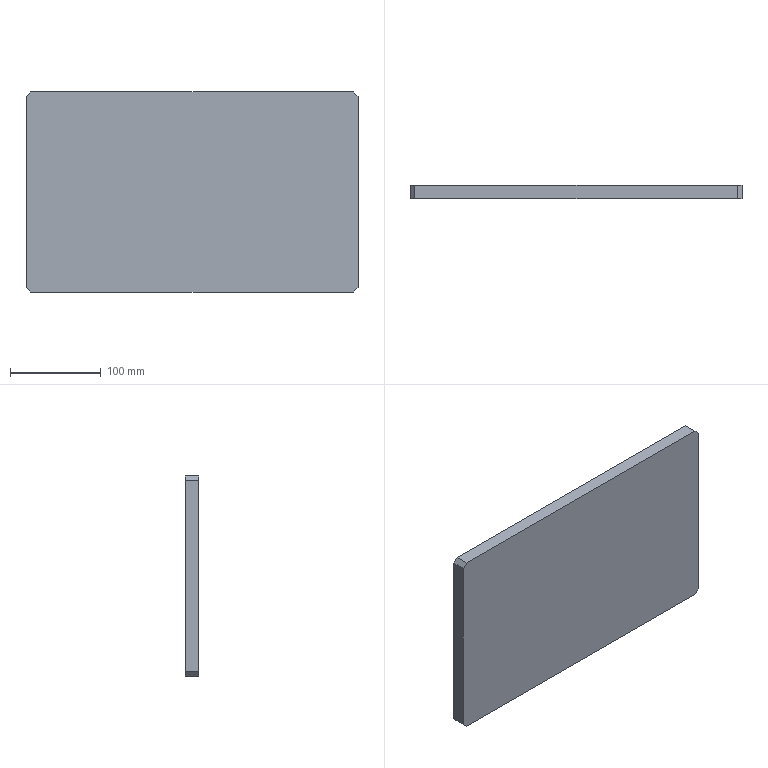Part | SolidWorks | features BaseBody 1 | 1 solid | 10 faces | box 365 x 15 x 220 mm | volume 1203750 mm3 | plane 10
STEP:
#1=CARTESIAN_POINT('',(360.,15.,-220.));
#2=VERTEX_POINT('',#1);
#3=CARTESIAN_POINT('',(365.,15.,-215.));
#4=VERTEX_POINT('',#3);
#5=CARTESIAN_POINT('',(360.,15.,-220.));
#6=DIRECTION('',(0.7071,0.,0.7071));
#7=VECTOR('',#6,1000.);
#8=LINE('',#5,#7);
#9=EDGE_CURVE('',#2,#4,#8,.T.);
#10=ORIENTED_EDGE('',*,*,#9,.F.);
#11=CARTESIAN_POINT('',(5.,15.,-220.));
#12=VERTEX_POINT('',#11);
#13=CARTESIAN_POINT('',(0.,15.,-220.));
#14=DIRECTION('',(1.,0.,0.));
#15=VECTOR('',#14,1000.);
#16=LINE('',#13,#15);
#17=EDGE_CURVE('',#12,#2,#16,.T.);
#18=ORIENTED_EDGE('',*,*,#17,.F.);
#19=CARTESIAN_POINT('',(0.,15.,-215.));
#20=VERTEX_POINT('',#19);
#21=CARTESIAN_POINT('',(0.,15.,-215.));
#22=DIRECTION('',(0.7071,0.,-0.7071));
#23=VECTOR('',#22,1000.);
#24=LINE('',#21,#23);
#25=EDGE_CURVE('',#20,#12,#24,.T.);
#26=ORIENTED_EDGE('',*,*,#25,.F.);
#27=CARTESIAN_POINT('',(0.,15.,-5.));
#28=VERTEX_POINT('',#27);
#29=CARTESIAN_POINT('',(0.,15.,0.));
#30=DIRECTION('',(0.,0.,-1.));
#31=VECTOR('',#30,1000.);
#32=LINE('',#29,#31);
#33=EDGE_CURVE('',#28,#20,#32,.T.);
#34=ORIENTED_EDGE('',*,*,#33,.F.);
#35=CARTESIAN_POINT('',(5.,15.,0.));
#36=VERTEX_POINT('',#35);
#37=CARTESIAN_POINT('',(5.,15.,0.));
#38=DIRECTION('',(-0.7071,0.,-0.7071));
#39=VECTOR('',#38,1000.);
#40=LINE('',#37,#39);
#41=EDGE_CURVE('',#36,#28,#40,.T.);
#42=ORIENTED_EDGE('',*,*,#41,.F.);
#43=CARTESIAN_POINT('',(360.,15.,0.));
#44=VERTEX_POINT('',#43);
#45=CARTESIAN_POINT('',(0.,15.,0.));
#46=DIRECTION('',(-1.,0.,0.));
#47=VECTOR('',#46,1000.);
#48=LINE('',#45,#47);
#49=EDGE_CURVE('',#44,#36,#48,.T.);
#50=ORIENTED_EDGE('',*,*,#49,.F.);
#51=CARTESIAN_POINT('',(365.,15.,-5.));
#52=VERTEX_POINT('',#51);
#53=CARTESIAN_POINT('',(365.,15.,-5.));
#54=DIRECTION('',(-0.7071,0.,0.7071));
#55=VECTOR('',#54,1000.);
#56=LINE('',#53,#55);
#57=EDGE_CURVE('',#52,#44,#56,.T.);
#58=ORIENTED_EDGE('',*,*,#57,.F.);
#59=CARTESIAN_POINT('',(365.,15.,0.));
#60=DIRECTION('',(0.,0.,1.));
#61=VECTOR('',#60,1000.);
#62=LINE('',#59,#61);
#63=EDGE_CURVE('',#4,#52,#62,.T.);
#64=ORIENTED_EDGE('',*,*,#63,.F.);
#65=EDGE_LOOP('',(#10,#18,#26,#34,#42,#50,#58,#64));
#66=FACE_OUTER_BOUND('',#65,.T.);
#67=CARTESIAN_POINT('',(0.,15.,0.));
#68=DIRECTION('',(0.,-1.,0.));
#69=DIRECTION('',(0.,0.,-1.));
#70=AXIS2_PLACEMENT_3D('',#67,#68,#69);
#71=PLANE('',#70);
#72=ADVANCED_FACE('',(#66),#71,.F.);
#73=CARTESIAN_POINT('',(365.,0.,-215.));
#74=VERTEX_POINT('',#73);
#75=CARTESIAN_POINT('',(365.,15.,-215.));
#76=DIRECTION('',(0.,-1.,0.));
#77=VECTOR('',#76,1000.);
#78=LINE('',#75,#77);
#79=EDGE_CURVE('',#4,#74,#78,.T.);
#80=ORIENTED_EDGE('',*,*,#79,.F.);
#81=ORIENTED_EDGE('',*,*,#63,.T.);
#82=CARTESIAN_POINT('',(365.,0.,-5.));
#83=VERTEX_POINT('',#82);
#84=CARTESIAN_POINT('',(365.,15.,-5.));
#85=DIRECTION('',(0.,1.,0.));
#86=VECTOR('',#85,1000.);
#87=LINE('',#84,#86);
#88=EDGE_CURVE('',#83,#52,#87,.T.);
#89=ORIENTED_EDGE('',*,*,#88,.F.);
#90=CARTESIAN_POINT('',(365.,0.,0.));
#91=DIRECTION('',(0.,0.,1.));
#92=VECTOR('',#91,1000.);
#93=LINE('',#90,#92);
#94=EDGE_CURVE('',#74,#83,#93,.T.);
#95=ORIENTED_EDGE('',*,*,#94,.F.);
#96=EDGE_LOOP('',(#80,#81,#89,#95));
#97=FACE_OUTER_BOUND('',#96,.T.);
#98=CARTESIAN_POINT('',(365.,15.,0.));
#99=DIRECTION('',(-1.,0.,0.));
#100=DIRECTION('',(0.,0.,1.));
#101=AXIS2_PLACEMENT_3D('',#98,#99,#100);
#102=PLANE('',#101);
#103=ADVANCED_FACE('',(#97),#102,.F.);
#104=ORIENTED_EDGE('',*,*,#79,.T.);
#105=CARTESIAN_POINT('',(360.,0.,-220.));
#106=VERTEX_POINT('',#105);
#107=CARTESIAN_POINT('',(360.,0.,-220.));
#108=DIRECTION('',(0.7071,0.,0.7071));
#109=VECTOR('',#108,1000.);
#110=LINE('',#107,#109);
#111=EDGE_CURVE('',#106,#74,#110,.T.);
#112=ORIENTED_EDGE('',*,*,#111,.F.);
#113=CARTESIAN_POINT('',(360.,15.,-220.));
#114=DIRECTION('',(0.,-1.,0.));
#115=VECTOR('',#114,1000.);
#116=LINE('',#113,#115);
#117=EDGE_CURVE('',#2,#106,#116,.T.);
#118=ORIENTED_EDGE('',*,*,#117,.F.);
#119=ORIENTED_EDGE('',*,*,#9,.T.);
#120=EDGE_LOOP('',(#104,#112,#118,#119));
#121=FACE_OUTER_BOUND('',#120,.T.);
#122=CARTESIAN_POINT('',(360.,15.,-220.));
#123=DIRECTION('',(-0.7071,0.,0.7071));
#124=DIRECTION('',(0.7071,0.,0.7071));
#125=AXIS2_PLACEMENT_3D('',#122,#123,#124);
#126=PLANE('',#125);
#127=ADVANCED_FACE('',(#121),#126,.F.);
#128=ORIENTED_EDGE('',*,*,#117,.T.);
#129=CARTESIAN_POINT('',(5.,0.,-220.));
#130=VERTEX_POINT('',#129);
#131=CARTESIAN_POINT('',(0.,0.,-220.));
#132=DIRECTION('',(1.,0.,0.));
#133=VECTOR('',#132,1000.);
#134=LINE('',#131,#133);
#135=EDGE_CURVE('',#130,#106,#134,.T.);
#136=ORIENTED_EDGE('',*,*,#135,.F.);
#137=CARTESIAN_POINT('',(5.,15.,-220.));
#138=DIRECTION('',(0.,-1.,0.));
#139=VECTOR('',#138,1000.);
#140=LINE('',#137,#139);
#141=EDGE_CURVE('',#12,#130,#140,.T.);
#142=ORIENTED_EDGE('',*,*,#141,.F.);
#143=ORIENTED_EDGE('',*,*,#17,.T.);
#144=EDGE_LOOP('',(#128,#136,#142,#143));
#145=FACE_OUTER_BOUND('',#144,.T.);
#146=CARTESIAN_POINT('',(0.,15.,-220.));
#147=DIRECTION('',(0.,0.,1.));
#148=DIRECTION('',(1.,0.,0.));
#149=AXIS2_PLACEMENT_3D('',#146,#147,#148);
#150=PLANE('',#149);
#151=ADVANCED_FACE('',(#145),#150,.F.);
#152=ORIENTED_EDGE('',*,*,#141,.T.);
#153=CARTESIAN_POINT('',(0.,0.,-215.));
#154=VERTEX_POINT('',#153);
#155=CARTESIAN_POINT('',(0.,0.,-215.));
#156=DIRECTION('',(0.7071,0.,-0.7071));
#157=VECTOR('',#156,1000.);
#158=LINE('',#155,#157);
#159=EDGE_CURVE('',#154,#130,#158,.T.);
#160=ORIENTED_EDGE('',*,*,#159,.F.);
#161=CARTESIAN_POINT('',(0.,15.,-215.));
#162=DIRECTION('',(0.,-1.,0.));
#163=VECTOR('',#162,1000.);
#164=LINE('',#161,#163);
#165=EDGE_CURVE('',#20,#154,#164,.T.);
#166=ORIENTED_EDGE('',*,*,#165,.F.);
#167=ORIENTED_EDGE('',*,*,#25,.T.);
#168=EDGE_LOOP('',(#152,#160,#166,#167));
#169=FACE_OUTER_BOUND('',#168,.T.);
#170=CARTESIAN_POINT('',(0.,15.,-215.));
#171=DIRECTION('',(0.7071,0.,0.7071));
#172=DIRECTION('',(0.7071,0.,-0.7071));
#173=AXIS2_PLACEMENT_3D('',#170,#171,#172);
#174=PLANE('',#173);
#175=ADVANCED_FACE('',(#169),#174,.F.);
#176=ORIENTED_EDGE('',*,*,#165,.T.);
#177=CARTESIAN_POINT('',(0.,0.,-5.));
#178=VERTEX_POINT('',#177);
#179=CARTESIAN_POINT('',(0.,0.,0.));
#180=DIRECTION('',(0.,0.,-1.));
#181=VECTOR('',#180,1000.);
#182=LINE('',#179,#181);
#183=EDGE_CURVE('',#178,#154,#182,.T.);
#184=ORIENTED_EDGE('',*,*,#183,.F.);
#185=CARTESIAN_POINT('',(0.,15.,-5.));
#186=DIRECTION('',(0.,-1.,0.));
#187=VECTOR('',#186,1000.);
#188=LINE('',#185,#187);
#189=EDGE_CURVE('',#28,#178,#188,.T.);
#190=ORIENTED_EDGE('',*,*,#189,.F.);
#191=ORIENTED_EDGE('',*,*,#33,.T.);
#192=EDGE_LOOP('',(#176,#184,#190,#191));
#193=FACE_OUTER_BOUND('',#192,.T.);
#194=CARTESIAN_POINT('',(0.,15.,0.));
#195=DIRECTION('',(1.,0.,0.));
#196=DIRECTION('',(0.,0.,-1.));
#197=AXIS2_PLACEMENT_3D('',#194,#195,#196);
#198=PLANE('',#197);
#199=ADVANCED_FACE('',(#193),#198,.F.);
#200=ORIENTED_EDGE('',*,*,#189,.T.);
#201=CARTESIAN_POINT('',(5.,0.,0.));
#202=VERTEX_POINT('',#201);
#203=CARTESIAN_POINT('',(5.,0.,0.));
#204=DIRECTION('',(-0.7071,0.,-0.7071));
#205=VECTOR('',#204,1000.);
#206=LINE('',#203,#205);
#207=EDGE_CURVE('',#202,#178,#206,.T.);
#208=ORIENTED_EDGE('',*,*,#207,.F.);
#209=CARTESIAN_POINT('',(5.,15.,0.));
#210=DIRECTION('',(0.,-1.,0.));
#211=VECTOR('',#210,1000.);
#212=LINE('',#209,#211);
#213=EDGE_CURVE('',#36,#202,#212,.T.);
#214=ORIENTED_EDGE('',*,*,#213,.F.);
#215=ORIENTED_EDGE('',*,*,#41,.T.);
#216=EDGE_LOOP('',(#200,#208,#214,#215));
#217=FACE_OUTER_BOUND('',#216,.T.);
#218=CARTESIAN_POINT('',(5.,15.,0.));
#219=DIRECTION('',(0.7071,0.,-0.7071));
#220=DIRECTION('',(-0.7071,0.,-0.7071));
#221=AXIS2_PLACEMENT_3D('',#218,#219,#220);
#222=PLANE('',#221);
#223=ADVANCED_FACE('',(#217),#222,.F.);
#224=CARTESIAN_POINT('',(360.,0.,0.));
#225=VERTEX_POINT('',#224);
#226=CARTESIAN_POINT('',(360.,15.,0.));
#227=DIRECTION('',(0.,-1.,0.));
#228=VECTOR('',#227,1000.);
#229=LINE('',#226,#228);
#230=EDGE_CURVE('',#44,#225,#229,.T.);
#231=ORIENTED_EDGE('',*,*,#230,.F.);
#232=ORIENTED_EDGE('',*,*,#49,.T.);
#233=ORIENTED_EDGE('',*,*,#213,.T.);
#234=CARTESIAN_POINT('',(0.,0.,0.));
#235=DIRECTION('',(-1.,0.,0.));
#236=VECTOR('',#235,1000.);
#237=LINE('',#234,#236);
#238=EDGE_CURVE('',#225,#202,#237,.T.);
#239=ORIENTED_EDGE('',*,*,#238,.F.);
#240=EDGE_LOOP('',(#231,#232,#233,#239));
#241=FACE_OUTER_BOUND('',#240,.T.);
#242=CARTESIAN_POINT('',(0.,15.,0.));
#243=DIRECTION('',(0.,0.,-1.));
#244=DIRECTION('',(-1.,0.,0.));
#245=AXIS2_PLACEMENT_3D('',#242,#243,#244);
#246=PLANE('',#245);
#247=ADVANCED_FACE('',(#241),#246,.F.);
#248=ORIENTED_EDGE('',*,*,#230,.T.);
#249=CARTESIAN_POINT('',(365.,0.,-5.));
#250=DIRECTION('',(-0.7071,0.,0.7071));
#251=VECTOR('',#250,1000.);
#252=LINE('',#249,#251);
#253=EDGE_CURVE('',#83,#225,#252,.T.);
#254=ORIENTED_EDGE('',*,*,#253,.F.);
#255=ORIENTED_EDGE('',*,*,#88,.T.);
#256=ORIENTED_EDGE('',*,*,#57,.T.);
#257=EDGE_LOOP('',(#248,#254,#255,#256));
#258=FACE_OUTER_BOUND('',#257,.T.);
#259=CARTESIAN_POINT('',(365.,15.,-5.));
#260=DIRECTION('',(-0.7071,0.,-0.7071));
#261=DIRECTION('',(-0.7071,0.,0.7071));
#262=AXIS2_PLACEMENT_3D('',#259,#260,#261);
#263=PLANE('',#262);
#264=ADVANCED_FACE('',(#258),#263,.F.);
#265=ORIENTED_EDGE('',*,*,#183,.T.);
#266=ORIENTED_EDGE('',*,*,#159,.T.);
#267=ORIENTED_EDGE('',*,*,#135,.T.);
#268=ORIENTED_EDGE('',*,*,#111,.T.);
#269=ORIENTED_EDGE('',*,*,#94,.T.);
#270=ORIENTED_EDGE('',*,*,#253,.T.);
#271=ORIENTED_EDGE('',*,*,#238,.T.);
#272=ORIENTED_EDGE('',*,*,#207,.T.);
#273=EDGE_LOOP('',(#265,#266,#267,#268,#269,#270,#271,#272));
#274=FACE_OUTER_BOUND('',#273,.T.);
#275=CARTESIAN_POINT('',(0.,0.,0.));
#276=DIRECTION('',(0.,-1.,0.));
#277=DIRECTION('',(0.,0.,-1.));
#278=AXIS2_PLACEMENT_3D('',#275,#276,#277);
#279=PLANE('',#278);
#280=ADVANCED_FACE('',(#274),#279,.T.);
#281=CLOSED_SHELL('',(#72,#103,#127,#151,#175,#199,#223,#247,#264,#280));
#282=MANIFOLD_SOLID_BREP('',#281);
#283=CARTESIAN_POINT('',(0.,0.,0.));
#284=DIRECTION('',(0.,0.,1.));
#285=DIRECTION('',(1.,0.,0.));
#286=AXIS2_PLACEMENT_3D('',#283,#284,#285);
#287=(LENGTH_UNIT()NAMED_UNIT(*)SI_UNIT(.MILLI.,.METRE.));
#288=UNCERTAINTY_MEASURE_WITH_UNIT(LENGTH_MEASURE(0.00001),#287,'','');
#289=(NAMED_UNIT(*)PLANE_ANGLE_UNIT()SI_UNIT($,.RADIAN.));
#290=(NAMED_UNIT(*)SI_UNIT($,.STERADIAN.)SOLID_ANGLE_UNIT());
#291=(GEOMETRIC_REPRESENTATION_CONTEXT(3)GLOBAL_UNCERTAINTY_ASSIGNED_CONTEXT((#288))GLOBAL_UNIT_ASSIGNED_CONTEXT((#287,#289,#290))REPRESENTATION_CONTEXT('',''));
#292=ADVANCED_BREP_SHAPE_REPRESENTATION('',(#282,#286),#291);